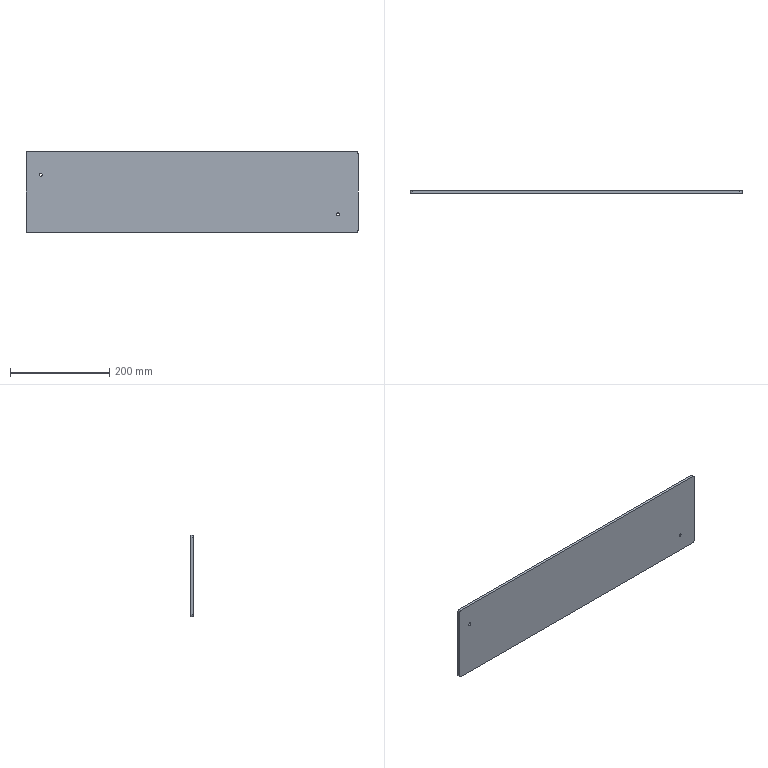Part | NX | 1 solid | 18 faces | box 670 x 5 x 164 mm | volume 549009 mm3 | cylinder 8 | plane 6 | cone 4 | commonest cylinder face diameters 6 x4 10 x4
STEP:
#1=CARTESIAN_POINT('',(759.,-747.5,-713.5));
#2=VERTEX_POINT('',#1);
#3=CARTESIAN_POINT('',(759.,-752.5,-713.5));
#4=VERTEX_POINT('',#3);
#5=CARTESIAN_POINT('',(759.,-752.5,-713.5));
#6=DIRECTION('',(0.,-1.,0.));
#7=VECTOR('',#6,1000.);
#8=LINE('',#5,#7);
#9=EDGE_CURVE('',#2,#4,#8,.T.);
#10=ORIENTED_EDGE('',*,*,#9,.T.);
#11=CARTESIAN_POINT('',(759.,-752.5,-867.5));
#12=VERTEX_POINT('',#11);
#13=CARTESIAN_POINT('',(759.,-752.5,-834.161));
#14=DIRECTION('',(0.,0.,-1.));
#15=VECTOR('',#14,1000.);
#16=LINE('',#13,#15);
#17=EDGE_CURVE('',#4,#12,#16,.T.);
#18=ORIENTED_EDGE('',*,*,#17,.T.);
#19=CARTESIAN_POINT('',(759.,-747.5,-867.5));
#20=VERTEX_POINT('',#19);
#21=CARTESIAN_POINT('',(759.,-752.5,-867.5));
#22=DIRECTION('',(0.,-1.,0.));
#23=VECTOR('',#22,1000.);
#24=LINE('',#21,#23);
#25=EDGE_CURVE('',#20,#12,#24,.T.);
#26=ORIENTED_EDGE('',*,*,#25,.F.);
#27=CARTESIAN_POINT('',(759.,-747.5,-834.161));
#28=DIRECTION('',(0.,0.,1.));
#29=VECTOR('',#28,1000.);
#30=LINE('',#27,#29);
#31=EDGE_CURVE('',#20,#2,#30,.T.);
#32=ORIENTED_EDGE('',*,*,#31,.T.);
#33=EDGE_LOOP('',(#10,#18,#26,#32));
#34=FACE_BOUND('',#33,.T.);
#35=CARTESIAN_POINT('',(759.,-752.5,-872.5));
#36=DIRECTION('',(1.,0.,0.));
#37=DIRECTION('',(0.,1.,0.));
#38=AXIS2_PLACEMENT_3D('',#35,#36,#37);
#39=PLANE('',#38);
#40=ADVANCED_FACE('',(#34),#39,.T.);
#41=CARTESIAN_POINT('',(94.,-752.5,-872.5));
#42=VERTEX_POINT('',#41);
#43=CARTESIAN_POINT('',(94.,-747.5,-872.5));
#44=VERTEX_POINT('',#43);
#45=CARTESIAN_POINT('',(94.,-752.5,-872.5));
#46=DIRECTION('',(0.,1.,0.));
#47=VECTOR('',#46,1000.);
#48=LINE('',#45,#47);
#49=EDGE_CURVE('',#42,#44,#48,.T.);
#50=ORIENTED_EDGE('',*,*,#49,.T.);
#51=CARTESIAN_POINT('',(754.,-747.5,-872.5));
#52=VERTEX_POINT('',#51);
#53=CARTESIAN_POINT('',(456.886,-747.5,-872.5));
#54=DIRECTION('',(1.,0.,0.));
#55=VECTOR('',#54,1000.);
#56=LINE('',#53,#55);
#57=EDGE_CURVE('',#44,#52,#56,.T.);
#58=ORIENTED_EDGE('',*,*,#57,.T.);
#59=CARTESIAN_POINT('',(754.,-752.5,-872.5));
#60=VERTEX_POINT('',#59);
#61=CARTESIAN_POINT('',(754.,-752.5,-872.5));
#62=DIRECTION('',(0.,-1.,0.));
#63=VECTOR('',#62,1000.);
#64=LINE('',#61,#63);
#65=EDGE_CURVE('',#52,#60,#64,.T.);
#66=ORIENTED_EDGE('',*,*,#65,.T.);
#67=CARTESIAN_POINT('',(456.886,-752.5,-872.5));
#68=DIRECTION('',(1.,0.,0.));
#69=VECTOR('',#68,1000.);
#70=LINE('',#67,#69);
#71=EDGE_CURVE('',#42,#60,#70,.T.);
#72=ORIENTED_EDGE('',*,*,#71,.F.);
#73=EDGE_LOOP('',(#50,#58,#66,#72));
#74=FACE_BOUND('',#73,.T.);
#75=CARTESIAN_POINT('',(94.,-752.5,-872.5));
#76=DIRECTION('',(0.,0.,-1.));
#77=DIRECTION('',(0.,-1.,0.));
#78=AXIS2_PLACEMENT_3D('',#75,#76,#77);
#79=PLANE('',#78);
#80=ADVANCED_FACE('',(#74),#79,.T.);
#81=CARTESIAN_POINT('',(89.,-747.5,-713.5));
#82=VERTEX_POINT('',#81);
#83=CARTESIAN_POINT('',(89.,-752.5,-713.5));
#84=VERTEX_POINT('',#83);
#85=CARTESIAN_POINT('',(89.,-752.5,-713.5));
#86=DIRECTION('',(0.,-1.,0.));
#87=VECTOR('',#86,1000.);
#88=LINE('',#85,#87);
#89=EDGE_CURVE('',#82,#84,#88,.T.);
#90=ORIENTED_EDGE('',*,*,#89,.F.);
#91=CARTESIAN_POINT('',(89.,-747.5,-867.5));
#92=VERTEX_POINT('',#91);
#93=CARTESIAN_POINT('',(89.,-747.5,-834.161));
#94=DIRECTION('',(0.,0.,-1.));
#95=VECTOR('',#94,1000.);
#96=LINE('',#93,#95);
#97=EDGE_CURVE('',#82,#92,#96,.T.);
#98=ORIENTED_EDGE('',*,*,#97,.T.);
#99=CARTESIAN_POINT('',(89.,-752.5,-867.5));
#100=VERTEX_POINT('',#99);
#101=CARTESIAN_POINT('',(89.,-752.5,-867.5));
#102=DIRECTION('',(0.,1.,0.));
#103=VECTOR('',#102,1000.);
#104=LINE('',#101,#103);
#105=EDGE_CURVE('',#100,#92,#104,.T.);
#106=ORIENTED_EDGE('',*,*,#105,.F.);
#107=CARTESIAN_POINT('',(89.,-752.5,-834.161));
#108=DIRECTION('',(0.,0.,1.));
#109=VECTOR('',#108,1000.);
#110=LINE('',#107,#109);
#111=EDGE_CURVE('',#100,#84,#110,.T.);
#112=ORIENTED_EDGE('',*,*,#111,.T.);
#113=EDGE_LOOP('',(#90,#98,#106,#112));
#114=FACE_BOUND('',#113,.T.);
#115=CARTESIAN_POINT('',(89.,-752.5,-718.5));
#116=DIRECTION('',(-1.,0.,0.));
#117=DIRECTION('',(0.,0.,1.));
#118=AXIS2_PLACEMENT_3D('',#115,#116,#117);
#119=PLANE('',#118);
#120=ADVANCED_FACE('',(#114),#119,.T.);
#121=CARTESIAN_POINT('',(94.,-752.5,-708.5));
#122=VERTEX_POINT('',#121);
#123=CARTESIAN_POINT('',(754.,-752.5,-708.5));
#124=VERTEX_POINT('',#123);
#125=CARTESIAN_POINT('',(456.886,-752.5,-708.5));
#126=DIRECTION('',(1.,0.,0.));
#127=VECTOR('',#126,1000.);
#128=LINE('',#125,#127);
#129=EDGE_CURVE('',#122,#124,#128,.T.);
#130=ORIENTED_EDGE('',*,*,#129,.T.);
#131=CARTESIAN_POINT('',(754.,-747.5,-708.5));
#132=VERTEX_POINT('',#131);
#133=CARTESIAN_POINT('',(754.,-752.5,-708.5));
#134=DIRECTION('',(0.,-1.,0.));
#135=VECTOR('',#134,1000.);
#136=LINE('',#133,#135);
#137=EDGE_CURVE('',#132,#124,#136,.T.);
#138=ORIENTED_EDGE('',*,*,#137,.F.);
#139=CARTESIAN_POINT('',(94.,-747.5,-708.5));
#140=VERTEX_POINT('',#139);
#141=CARTESIAN_POINT('',(456.886,-747.5,-708.5));
#142=DIRECTION('',(-1.,0.,0.));
#143=VECTOR('',#142,1000.);
#144=LINE('',#141,#143);
#145=EDGE_CURVE('',#132,#140,#144,.T.);
#146=ORIENTED_EDGE('',*,*,#145,.T.);
#147=CARTESIAN_POINT('',(94.,-752.5,-708.5));
#148=DIRECTION('',(0.,-1.,0.));
#149=VECTOR('',#148,1000.);
#150=LINE('',#147,#149);
#151=EDGE_CURVE('',#140,#122,#150,.T.);
#152=ORIENTED_EDGE('',*,*,#151,.T.);
#153=EDGE_LOOP('',(#130,#138,#146,#152));
#154=FACE_BOUND('',#153,.T.);
#155=CARTESIAN_POINT('',(754.,-752.5,-708.5));
#156=DIRECTION('',(0.,0.,1.));
#157=DIRECTION('',(1.,0.,0.));
#158=AXIS2_PLACEMENT_3D('',#155,#156,#157);
#159=PLANE('',#158);
#160=ADVANCED_FACE('',(#154),#159,.T.);
#161=ORIENTED_EDGE('',*,*,#25,.T.);
#162=CARTESIAN_POINT('',(754.,-752.5,-867.5));
#163=DIRECTION('',(0.,-1.,0.));
#164=DIRECTION('',(1.,0.,0.));
#165=AXIS2_PLACEMENT_3D('',#162,#163,#164);
#166=CIRCLE('',#165,5.);
#167=EDGE_CURVE('',#60,#12,#166,.T.);
#168=ORIENTED_EDGE('',*,*,#167,.F.);
#169=ORIENTED_EDGE('',*,*,#65,.F.);
#170=CARTESIAN_POINT('',(754.,-747.5,-867.5));
#171=DIRECTION('',(0.,-1.,0.));
#172=DIRECTION('',(1.,0.,0.));
#173=AXIS2_PLACEMENT_3D('',#170,#171,#172);
#174=CIRCLE('',#173,5.);
#175=EDGE_CURVE('',#52,#20,#174,.T.);
#176=ORIENTED_EDGE('',*,*,#175,.T.);
#177=EDGE_LOOP('',(#161,#168,#169,#176));
#178=FACE_BOUND('',#177,.T.);
#179=CARTESIAN_POINT('',(754.,-752.5,-867.5));
#180=DIRECTION('',(0.,-1.,0.));
#181=DIRECTION('',(1.,0.,0.));
#182=AXIS2_PLACEMENT_3D('',#179,#180,#181);
#183=CYLINDRICAL_SURFACE('',#182,5.);
#184=ADVANCED_FACE('',(#178),#183,.T.);
#185=ORIENTED_EDGE('',*,*,#9,.F.);
#186=CARTESIAN_POINT('',(754.,-747.5,-713.5));
#187=DIRECTION('',(0.,-1.,0.));
#188=DIRECTION('',(1.,0.,0.));
#189=AXIS2_PLACEMENT_3D('',#186,#187,#188);
#190=CIRCLE('',#189,5.);
#191=EDGE_CURVE('',#2,#132,#190,.T.);
#192=ORIENTED_EDGE('',*,*,#191,.T.);
#193=ORIENTED_EDGE('',*,*,#137,.T.);
#194=CARTESIAN_POINT('',(754.,-752.5,-713.5));
#195=DIRECTION('',(0.,-1.,0.));
#196=DIRECTION('',(1.,0.,0.));
#197=AXIS2_PLACEMENT_3D('',#194,#195,#196);
#198=CIRCLE('',#197,5.);
#199=EDGE_CURVE('',#4,#124,#198,.T.);
#200=ORIENTED_EDGE('',*,*,#199,.F.);
#201=EDGE_LOOP('',(#185,#192,#193,#200));
#202=FACE_BOUND('',#201,.T.);
#203=CARTESIAN_POINT('',(754.,-752.5,-713.5));
#204=DIRECTION('',(0.,-1.,0.));
#205=DIRECTION('',(1.,0.,0.));
#206=AXIS2_PLACEMENT_3D('',#203,#204,#205);
#207=CYLINDRICAL_SURFACE('',#206,5.);
#208=ADVANCED_FACE('',(#202),#207,.T.);
#209=ORIENTED_EDGE('',*,*,#89,.T.);
#210=CARTESIAN_POINT('',(94.,-752.5,-713.5));
#211=DIRECTION('',(0.,-1.,0.));
#212=DIRECTION('',(1.,0.,0.));
#213=AXIS2_PLACEMENT_3D('',#210,#211,#212);
#214=CIRCLE('',#213,5.);
#215=EDGE_CURVE('',#122,#84,#214,.T.);
#216=ORIENTED_EDGE('',*,*,#215,.F.);
#217=ORIENTED_EDGE('',*,*,#151,.F.);
#218=CARTESIAN_POINT('',(94.,-747.5,-713.5));
#219=DIRECTION('',(0.,-1.,0.));
#220=DIRECTION('',(1.,0.,0.));
#221=AXIS2_PLACEMENT_3D('',#218,#219,#220);
#222=CIRCLE('',#221,5.);
#223=EDGE_CURVE('',#140,#82,#222,.T.);
#224=ORIENTED_EDGE('',*,*,#223,.T.);
#225=EDGE_LOOP('',(#209,#216,#217,#224));
#226=FACE_BOUND('',#225,.T.);
#227=CARTESIAN_POINT('',(94.,-752.5,-713.5));
#228=DIRECTION('',(0.,-1.,0.));
#229=DIRECTION('',(1.,0.,0.));
#230=AXIS2_PLACEMENT_3D('',#227,#228,#229);
#231=CYLINDRICAL_SURFACE('',#230,5.);
#232=ADVANCED_FACE('',(#226),#231,.T.);
#233=ORIENTED_EDGE('',*,*,#49,.F.);
#234=CARTESIAN_POINT('',(94.,-752.5,-867.5));
#235=DIRECTION('',(0.,1.,0.));
#236=DIRECTION('',(-1.,0.,0.));
#237=AXIS2_PLACEMENT_3D('',#234,#235,#236);
#238=CIRCLE('',#237,5.);
#239=EDGE_CURVE('',#42,#100,#238,.T.);
#240=ORIENTED_EDGE('',*,*,#239,.T.);
#241=ORIENTED_EDGE('',*,*,#105,.T.);
#242=CARTESIAN_POINT('',(94.,-747.5,-867.5));
#243=DIRECTION('',(0.,1.,0.));
#244=DIRECTION('',(-1.,0.,0.));
#245=AXIS2_PLACEMENT_3D('',#242,#243,#244);
#246=CIRCLE('',#245,5.);
#247=EDGE_CURVE('',#44,#92,#246,.T.);
#248=ORIENTED_EDGE('',*,*,#247,.F.);
#249=EDGE_LOOP('',(#233,#240,#241,#248));
#250=FACE_BOUND('',#249,.T.);
#251=CARTESIAN_POINT('',(94.,-752.5,-867.5));
#252=DIRECTION('',(0.,1.,0.));
#253=DIRECTION('',(-1.,0.,0.));
#254=AXIS2_PLACEMENT_3D('',#251,#252,#253);
#255=CYLINDRICAL_SURFACE('',#254,5.);
#256=ADVANCED_FACE('',(#250),#255,.T.);
#257=ORIENTED_EDGE('',*,*,#97,.F.);
#258=ORIENTED_EDGE('',*,*,#223,.F.);
#259=ORIENTED_EDGE('',*,*,#145,.F.);
#260=ORIENTED_EDGE('',*,*,#191,.F.);
#261=ORIENTED_EDGE('',*,*,#31,.F.);
#262=ORIENTED_EDGE('',*,*,#175,.F.);
#263=ORIENTED_EDGE('',*,*,#57,.F.);
#264=ORIENTED_EDGE('',*,*,#247,.T.);
#265=EDGE_LOOP('',(#257,#258,#259,#260,#261,#262,#263,#264));
#266=FACE_BOUND('',#265,.T.);
#267=CARTESIAN_POINT('',(121.7,-747.5,-755.5));
#268=VERTEX_POINT('',#267);
#269=CARTESIAN_POINT('',(115.3,-747.5,-755.5));
#270=VERTEX_POINT('',#269);
#271=CARTESIAN_POINT('',(118.5,-747.5,-755.5));
#272=DIRECTION('',(0.,1.,0.));
#273=DIRECTION('',(-1.,0.,0.));
#274=AXIS2_PLACEMENT_3D('',#271,#272,#273);
#275=CIRCLE('',#274,3.2);
#276=EDGE_CURVE('',#268,#270,#275,.T.);
#277=ORIENTED_EDGE('',*,*,#276,.F.);
#278=CARTESIAN_POINT('',(118.5,-747.5,-755.5));
#279=DIRECTION('',(0.,1.,0.));
#280=DIRECTION('',(-1.,0.,0.));
#281=AXIS2_PLACEMENT_3D('',#278,#279,#280);
#282=CIRCLE('',#281,3.2);
#283=EDGE_CURVE('',#270,#268,#282,.T.);
#284=ORIENTED_EDGE('',*,*,#283,.F.);
#285=EDGE_LOOP('',(#277,#284));
#286=FACE_BOUND('',#285,.T.);
#287=CARTESIAN_POINT('',(721.7,-747.5,-835.5));
#288=VERTEX_POINT('',#287);
#289=CARTESIAN_POINT('',(715.3,-747.5,-835.5));
#290=VERTEX_POINT('',#289);
#291=CARTESIAN_POINT('',(718.5,-747.5,-835.5));
#292=DIRECTION('',(0.,1.,0.));
#293=DIRECTION('',(-1.,0.,0.));
#294=AXIS2_PLACEMENT_3D('',#291,#292,#293);
#295=CIRCLE('',#294,3.2);
#296=EDGE_CURVE('',#288,#290,#295,.T.);
#297=ORIENTED_EDGE('',*,*,#296,.F.);
#298=CARTESIAN_POINT('',(718.5,-747.5,-835.5));
#299=DIRECTION('',(0.,1.,0.));
#300=DIRECTION('',(-1.,0.,0.));
#301=AXIS2_PLACEMENT_3D('',#298,#299,#300);
#302=CIRCLE('',#301,3.2);
#303=EDGE_CURVE('',#290,#288,#302,.T.);
#304=ORIENTED_EDGE('',*,*,#303,.F.);
#305=EDGE_LOOP('',(#297,#304));
#306=FACE_BOUND('',#305,.T.);
#307=CARTESIAN_POINT('',(456.886,-747.5,-834.161));
#308=DIRECTION('',(0.,1.,0.));
#309=DIRECTION('',(1.,0.,0.));
#310=AXIS2_PLACEMENT_3D('',#307,#308,#309);
#311=PLANE('',#310);
#312=ADVANCED_FACE('',(#266,#286,#306),#311,.T.);
#313=CARTESIAN_POINT('',(721.5,-747.7,-835.5));
#314=VERTEX_POINT('',#313);
#315=CARTESIAN_POINT('',(715.5,-747.7,-835.5));
#316=VERTEX_POINT('',#315);
#317=CARTESIAN_POINT('',(718.5,-747.7,-835.5));
#318=DIRECTION('',(0.,1.,0.));
#319=DIRECTION('',(-1.,0.,0.));
#320=AXIS2_PLACEMENT_3D('',#317,#318,#319);
#321=CIRCLE('',#320,3.);
#322=EDGE_CURVE('',#314,#316,#321,.T.);
#323=ORIENTED_EDGE('',*,*,#322,.T.);
#324=CARTESIAN_POINT('',(715.5,-752.5,-835.5));
#325=VERTEX_POINT('',#324);
#326=CARTESIAN_POINT('',(715.5,-747.5,-835.5));
#327=DIRECTION('',(0.,1.,0.));
#328=VECTOR('',#327,1000.);
#329=LINE('',#326,#328);
#330=EDGE_CURVE('',#316,#325,#329,.F.);
#331=ORIENTED_EDGE('',*,*,#330,.T.);
#332=CARTESIAN_POINT('',(721.5,-752.5,-835.5));
#333=VERTEX_POINT('',#332);
#334=CARTESIAN_POINT('',(718.5,-752.5,-835.5));
#335=DIRECTION('',(0.,1.,0.));
#336=DIRECTION('',(-1.,0.,0.));
#337=AXIS2_PLACEMENT_3D('',#334,#335,#336);
#338=CIRCLE('',#337,3.);
#339=EDGE_CURVE('',#333,#325,#338,.T.);
#340=ORIENTED_EDGE('',*,*,#339,.F.);
#341=CARTESIAN_POINT('',(721.5,-747.5,-835.5));
#342=DIRECTION('',(0.,1.,0.));
#343=VECTOR('',#342,1000.);
#344=LINE('',#341,#343);
#345=EDGE_CURVE('',#314,#333,#344,.F.);
#346=ORIENTED_EDGE('',*,*,#345,.F.);
#347=EDGE_LOOP('',(#323,#331,#340,#346));
#348=FACE_BOUND('',#347,.T.);
#349=CARTESIAN_POINT('',(718.5,-747.5,-835.5));
#350=DIRECTION('',(0.,1.,0.));
#351=DIRECTION('',(-1.,0.,0.));
#352=AXIS2_PLACEMENT_3D('',#349,#350,#351);
#353=CYLINDRICAL_SURFACE('',#352,3.);
#354=ADVANCED_FACE('',(#348),#353,.F.);
#355=CARTESIAN_POINT('',(121.5,-747.7,-755.5));
#356=VERTEX_POINT('',#355);
#357=CARTESIAN_POINT('',(115.5,-747.7,-755.5));
#358=VERTEX_POINT('',#357);
#359=CARTESIAN_POINT('',(118.5,-747.7,-755.5));
#360=DIRECTION('',(0.,1.,0.));
#361=DIRECTION('',(-1.,0.,0.));
#362=AXIS2_PLACEMENT_3D('',#359,#360,#361);
#363=CIRCLE('',#362,3.);
#364=EDGE_CURVE('',#356,#358,#363,.T.);
#365=ORIENTED_EDGE('',*,*,#364,.F.);
#366=CARTESIAN_POINT('',(121.5,-747.7,-755.5));
#367=DIRECTION('',(0.7071,0.7071,0.));
#368=VECTOR('',#367,1000.);
#369=LINE('',#366,#368);
#370=EDGE_CURVE('',#268,#356,#369,.F.);
#371=ORIENTED_EDGE('',*,*,#370,.F.);
#372=ORIENTED_EDGE('',*,*,#276,.T.);
#373=CARTESIAN_POINT('',(115.5,-747.7,-755.5));
#374=DIRECTION('',(-0.7071,0.7071,0.));
#375=VECTOR('',#374,1000.);
#376=LINE('',#373,#375);
#377=EDGE_CURVE('',#270,#358,#376,.F.);
#378=ORIENTED_EDGE('',*,*,#377,.T.);
#379=EDGE_LOOP('',(#365,#371,#372,#378));
#380=FACE_BOUND('',#379,.T.);
#381=CARTESIAN_POINT('',(118.5,-747.7,-755.5));
#382=DIRECTION('',(0.,1.,0.));
#383=DIRECTION('',(-1.,0.,0.));
#384=AXIS2_PLACEMENT_3D('',#381,#382,#383);
#385=CONICAL_SURFACE('',#384,3.,0.7854);
#386=ADVANCED_FACE('',(#380),#385,.F.);
#387=ORIENTED_EDGE('',*,*,#364,.T.);
#388=CARTESIAN_POINT('',(115.5,-752.5,-755.5));
#389=VERTEX_POINT('',#388);
#390=CARTESIAN_POINT('',(115.5,-747.5,-755.5));
#391=DIRECTION('',(0.,1.,0.));
#392=VECTOR('',#391,1000.);
#393=LINE('',#390,#392);
#394=EDGE_CURVE('',#358,#389,#393,.F.);
#395=ORIENTED_EDGE('',*,*,#394,.T.);
#396=CARTESIAN_POINT('',(121.5,-752.5,-755.5));
#397=VERTEX_POINT('',#396);
#398=CARTESIAN_POINT('',(118.5,-752.5,-755.5));
#399=DIRECTION('',(0.,1.,0.));
#400=DIRECTION('',(-1.,0.,0.));
#401=AXIS2_PLACEMENT_3D('',#398,#399,#400);
#402=CIRCLE('',#401,3.);
#403=EDGE_CURVE('',#397,#389,#402,.T.);
#404=ORIENTED_EDGE('',*,*,#403,.F.);
#405=CARTESIAN_POINT('',(121.5,-747.5,-755.5));
#406=DIRECTION('',(0.,1.,0.));
#407=VECTOR('',#406,1000.);
#408=LINE('',#405,#407);
#409=EDGE_CURVE('',#356,#397,#408,.F.);
#410=ORIENTED_EDGE('',*,*,#409,.F.);
#411=EDGE_LOOP('',(#387,#395,#404,#410));
#412=FACE_BOUND('',#411,.T.);
#413=CARTESIAN_POINT('',(118.5,-747.5,-755.5));
#414=DIRECTION('',(0.,1.,0.));
#415=DIRECTION('',(-1.,0.,0.));
#416=AXIS2_PLACEMENT_3D('',#413,#414,#415);
#417=CYLINDRICAL_SURFACE('',#416,3.);
#418=ADVANCED_FACE('',(#412),#417,.F.);
#419=ORIENTED_EDGE('',*,*,#322,.F.);
#420=CARTESIAN_POINT('',(721.5,-747.7,-835.5));
#421=DIRECTION('',(0.7071,0.7071,0.));
#422=VECTOR('',#421,1000.);
#423=LINE('',#420,#422);
#424=EDGE_CURVE('',#288,#314,#423,.F.);
#425=ORIENTED_EDGE('',*,*,#424,.F.);
#426=ORIENTED_EDGE('',*,*,#296,.T.);
#427=CARTESIAN_POINT('',(715.5,-747.7,-835.5));
#428=DIRECTION('',(-0.7071,0.7071,0.));
#429=VECTOR('',#428,1000.);
#430=LINE('',#427,#429);
#431=EDGE_CURVE('',#290,#316,#430,.F.);
#432=ORIENTED_EDGE('',*,*,#431,.T.);
#433=EDGE_LOOP('',(#419,#425,#426,#432));
#434=FACE_BOUND('',#433,.T.);
#435=CARTESIAN_POINT('',(718.5,-747.7,-835.5));
#436=DIRECTION('',(0.,1.,0.));
#437=DIRECTION('',(-1.,0.,0.));
#438=AXIS2_PLACEMENT_3D('',#435,#436,#437);
#439=CONICAL_SURFACE('',#438,3.,0.7854);
#440=ADVANCED_FACE('',(#434),#439,.F.);
#441=ORIENTED_EDGE('',*,*,#377,.F.);
#442=ORIENTED_EDGE('',*,*,#283,.T.);
#443=ORIENTED_EDGE('',*,*,#370,.T.);
#444=CARTESIAN_POINT('',(118.5,-747.7,-755.5));
#445=DIRECTION('',(0.,1.,0.));
#446=DIRECTION('',(-1.,0.,0.));
#447=AXIS2_PLACEMENT_3D('',#444,#445,#446);
#448=CIRCLE('',#447,3.);
#449=EDGE_CURVE('',#358,#356,#448,.T.);
#450=ORIENTED_EDGE('',*,*,#449,.F.);
#451=EDGE_LOOP('',(#441,#442,#443,#450));
#452=FACE_BOUND('',#451,.T.);
#453=CARTESIAN_POINT('',(118.5,-747.7,-755.5));
#454=DIRECTION('',(0.,1.,0.));
#455=DIRECTION('',(-1.,0.,0.));
#456=AXIS2_PLACEMENT_3D('',#453,#454,#455);
#457=CONICAL_SURFACE('',#456,3.,0.7854);
#458=ADVANCED_FACE('',(#452),#457,.F.);
#459=ORIENTED_EDGE('',*,*,#394,.F.);
#460=ORIENTED_EDGE('',*,*,#449,.T.);
#461=ORIENTED_EDGE('',*,*,#409,.T.);
#462=CARTESIAN_POINT('',(118.5,-752.5,-755.5));
#463=DIRECTION('',(0.,1.,0.));
#464=DIRECTION('',(-1.,0.,0.));
#465=AXIS2_PLACEMENT_3D('',#462,#463,#464);
#466=CIRCLE('',#465,3.);
#467=EDGE_CURVE('',#389,#397,#466,.T.);
#468=ORIENTED_EDGE('',*,*,#467,.F.);
#469=EDGE_LOOP('',(#459,#460,#461,#468));
#470=FACE_BOUND('',#469,.T.);
#471=CARTESIAN_POINT('',(118.5,-747.5,-755.5));
#472=DIRECTION('',(0.,1.,0.));
#473=DIRECTION('',(-1.,0.,0.));
#474=AXIS2_PLACEMENT_3D('',#471,#472,#473);
#475=CYLINDRICAL_SURFACE('',#474,3.);
#476=ADVANCED_FACE('',(#470),#475,.F.);
#477=ORIENTED_EDGE('',*,*,#330,.F.);
#478=CARTESIAN_POINT('',(718.5,-747.7,-835.5));
#479=DIRECTION('',(0.,1.,0.));
#480=DIRECTION('',(-1.,0.,0.));
#481=AXIS2_PLACEMENT_3D('',#478,#479,#480);
#482=CIRCLE('',#481,3.);
#483=EDGE_CURVE('',#316,#314,#482,.T.);
#484=ORIENTED_EDGE('',*,*,#483,.T.);
#485=ORIENTED_EDGE('',*,*,#345,.T.);
#486=CARTESIAN_POINT('',(718.5,-752.5,-835.5));
#487=DIRECTION('',(0.,1.,0.));
#488=DIRECTION('',(-1.,0.,0.));
#489=AXIS2_PLACEMENT_3D('',#486,#487,#488);
#490=CIRCLE('',#489,3.);
#491=EDGE_CURVE('',#325,#333,#490,.T.);
#492=ORIENTED_EDGE('',*,*,#491,.F.);
#493=EDGE_LOOP('',(#477,#484,#485,#492));
#494=FACE_BOUND('',#493,.T.);
#495=CARTESIAN_POINT('',(718.5,-747.5,-835.5));
#496=DIRECTION('',(0.,1.,0.));
#497=DIRECTION('',(-1.,0.,0.));
#498=AXIS2_PLACEMENT_3D('',#495,#496,#497);
#499=CYLINDRICAL_SURFACE('',#498,3.);
#500=ADVANCED_FACE('',(#494),#499,.F.);
#501=ORIENTED_EDGE('',*,*,#431,.F.);
#502=ORIENTED_EDGE('',*,*,#303,.T.);
#503=ORIENTED_EDGE('',*,*,#424,.T.);
#504=ORIENTED_EDGE('',*,*,#483,.F.);
#505=EDGE_LOOP('',(#501,#502,#503,#504));
#506=FACE_BOUND('',#505,.T.);
#507=CARTESIAN_POINT('',(718.5,-747.7,-835.5));
#508=DIRECTION('',(0.,1.,0.));
#509=DIRECTION('',(-1.,0.,0.));
#510=AXIS2_PLACEMENT_3D('',#507,#508,#509);
#511=CONICAL_SURFACE('',#510,3.,0.7854);
#512=ADVANCED_FACE('',(#506),#511,.F.);
#513=ORIENTED_EDGE('',*,*,#71,.T.);
#514=ORIENTED_EDGE('',*,*,#167,.T.);
#515=ORIENTED_EDGE('',*,*,#17,.F.);
#516=ORIENTED_EDGE('',*,*,#199,.T.);
#517=ORIENTED_EDGE('',*,*,#129,.F.);
#518=ORIENTED_EDGE('',*,*,#215,.T.);
#519=ORIENTED_EDGE('',*,*,#111,.F.);
#520=ORIENTED_EDGE('',*,*,#239,.F.);
#521=EDGE_LOOP('',(#513,#514,#515,#516,#517,#518,#519,#520));
#522=FACE_BOUND('',#521,.T.);
#523=ORIENTED_EDGE('',*,*,#339,.T.);
#524=ORIENTED_EDGE('',*,*,#491,.T.);
#525=EDGE_LOOP('',(#523,#524));
#526=FACE_BOUND('',#525,.T.);
#527=ORIENTED_EDGE('',*,*,#403,.T.);
#528=ORIENTED_EDGE('',*,*,#467,.T.);
#529=EDGE_LOOP('',(#527,#528));
#530=FACE_BOUND('',#529,.T.);
#531=CARTESIAN_POINT('',(456.886,-752.5,-834.161));
#532=DIRECTION('',(0.,1.,0.));
#533=DIRECTION('',(1.,0.,0.));
#534=AXIS2_PLACEMENT_3D('',#531,#532,#533);
#535=PLANE('',#534);
#536=ADVANCED_FACE('',(#522,#526,#530),#535,.F.);
#537=CLOSED_SHELL('',(#40,#80,#120,#160,#184,#208,#232,#256,#312,#354,#386,#418,#440,#458,#476,#500,#512,#536));
#538=MANIFOLD_SOLID_BREP('',#537);
#539=(LENGTH_UNIT()NAMED_UNIT(*)SI_UNIT(.MILLI.,.METRE.));
#540=UNCERTAINTY_MEASURE_WITH_UNIT(LENGTH_MEASURE(0.00001),#539,'','');
#541=(NAMED_UNIT(*)PLANE_ANGLE_UNIT()SI_UNIT($,.RADIAN.));
#542=(NAMED_UNIT(*)SI_UNIT($,.STERADIAN.)SOLID_ANGLE_UNIT());
#543=(GEOMETRIC_REPRESENTATION_CONTEXT(3)GLOBAL_UNCERTAINTY_ASSIGNED_CONTEXT((#540))GLOBAL_UNIT_ASSIGNED_CONTEXT((#539,#541,#542))REPRESENTATION_CONTEXT('',''));
#544=ADVANCED_BREP_SHAPE_REPRESENTATION('',(#538),#543);